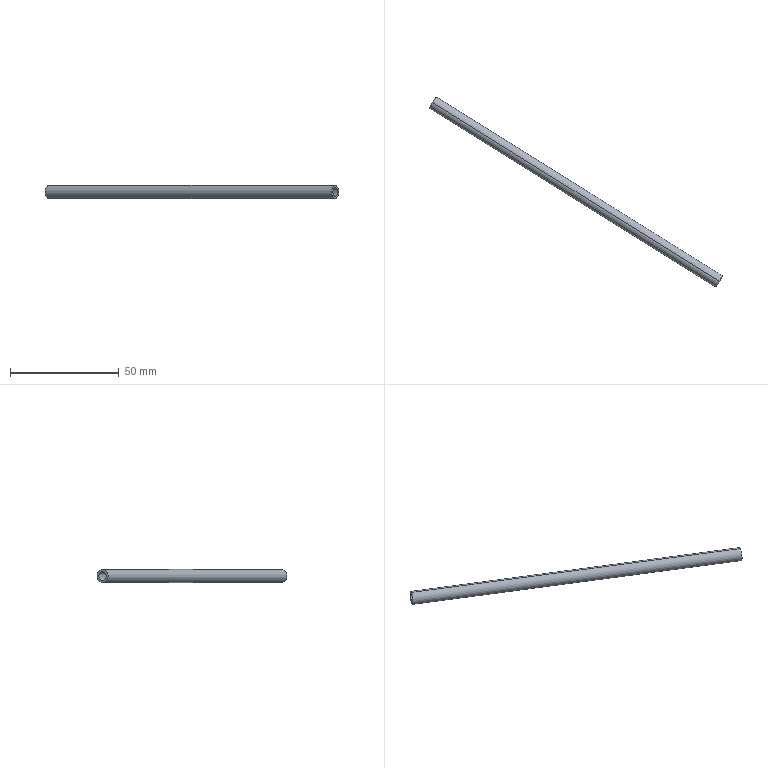Part | SolidWorks | features BaseBody 1 | 1 solid | 6 faces | box 134.627 x 87.226 x 6 mm | volume 2435 mm3 | cylinder 4 | plane 2 | commonest cylinder face diameters 4 x2 6 x2
STEP:
#1=CARTESIAN_POINT('',(-187.965,151.587,-231.5));
#2=VERTEX_POINT('',#1);
#3=CARTESIAN_POINT('',(-187.965,151.587,-235.5));
#4=VERTEX_POINT('',#3);
#5=CARTESIAN_POINT('',(-187.965,151.587,-233.5));
#6=DIRECTION('',(0.848,-0.5299,0.));
#7=DIRECTION('',(-0.5299,-0.848,0.));
#8=AXIS2_PLACEMENT_3D('',#5,#6,#7);
#9=CIRCLE('',#8,2.);
#10=EDGE_CURVE('',#2,#4,#9,.T.);
#11=ORIENTED_EDGE('',*,*,#10,.F.);
#12=CARTESIAN_POINT('',(-56.517,69.449,-231.5));
#13=VERTEX_POINT('',#12);
#14=CARTESIAN_POINT('',(-56.517,69.449,-231.5));
#15=DIRECTION('',(0.848,-0.5299,0.));
#16=VECTOR('',#15,1000.);
#17=LINE('',#14,#16);
#18=EDGE_CURVE('',#2,#13,#17,.T.);
#19=ORIENTED_EDGE('',*,*,#18,.T.);
#20=CARTESIAN_POINT('',(-56.517,69.449,-235.5));
#21=VERTEX_POINT('',#20);
#22=CARTESIAN_POINT('',(-56.517,69.449,-233.5));
#23=DIRECTION('',(0.848,-0.5299,0.));
#24=DIRECTION('',(0.,0.,-1.));
#25=AXIS2_PLACEMENT_3D('',#22,#23,#24);
#26=CIRCLE('',#25,2.);
#27=EDGE_CURVE('',#13,#21,#26,.T.);
#28=ORIENTED_EDGE('',*,*,#27,.T.);
#29=CARTESIAN_POINT('',(-56.517,69.449,-235.5));
#30=DIRECTION('',(0.848,-0.5299,0.));
#31=VECTOR('',#30,1000.);
#32=LINE('',#29,#31);
#33=EDGE_CURVE('',#4,#21,#32,.T.);
#34=ORIENTED_EDGE('',*,*,#33,.F.);
#35=EDGE_LOOP('',(#11,#19,#28,#34));
#36=FACE_OUTER_BOUND('',#35,.T.);
#37=CARTESIAN_POINT('',(-56.517,69.449,-233.5));
#38=DIRECTION('',(0.848,-0.5299,0.));
#39=DIRECTION('',(0.,0.,-1.));
#40=AXIS2_PLACEMENT_3D('',#37,#38,#39);
#41=CYLINDRICAL_SURFACE('',#40,2.);
#42=ADVANCED_FACE('',(#36),#41,.F.);
#43=CARTESIAN_POINT('',(-187.965,151.587,-236.5));
#44=VERTEX_POINT('',#43);
#45=CARTESIAN_POINT('',(-187.965,151.587,-230.5));
#46=VERTEX_POINT('',#45);
#47=CARTESIAN_POINT('',(-187.965,151.587,-233.5));
#48=DIRECTION('',(0.848,-0.5299,0.));
#49=DIRECTION('',(-0.5299,-0.848,0.));
#50=AXIS2_PLACEMENT_3D('',#47,#48,#49);
#51=CIRCLE('',#50,3.);
#52=EDGE_CURVE('',#44,#46,#51,.T.);
#53=ORIENTED_EDGE('',*,*,#52,.T.);
#54=CARTESIAN_POINT('',(-56.517,69.449,-230.5));
#55=VERTEX_POINT('',#54);
#56=CARTESIAN_POINT('',(-56.517,69.449,-230.5));
#57=DIRECTION('',(0.848,-0.5299,0.));
#58=VECTOR('',#57,1000.);
#59=LINE('',#56,#58);
#60=EDGE_CURVE('',#46,#55,#59,.T.);
#61=ORIENTED_EDGE('',*,*,#60,.T.);
#62=CARTESIAN_POINT('',(-56.517,69.449,-236.5));
#63=VERTEX_POINT('',#62);
#64=CARTESIAN_POINT('',(-56.517,69.449,-233.5));
#65=DIRECTION('',(0.848,-0.5299,0.));
#66=DIRECTION('',(0.,0.,-1.));
#67=AXIS2_PLACEMENT_3D('',#64,#65,#66);
#68=CIRCLE('',#67,3.);
#69=EDGE_CURVE('',#63,#55,#68,.T.);
#70=ORIENTED_EDGE('',*,*,#69,.F.);
#71=CARTESIAN_POINT('',(-56.517,69.449,-236.5));
#72=DIRECTION('',(0.848,-0.5299,0.));
#73=VECTOR('',#72,1000.);
#74=LINE('',#71,#73);
#75=EDGE_CURVE('',#44,#63,#74,.T.);
#76=ORIENTED_EDGE('',*,*,#75,.F.);
#77=EDGE_LOOP('',(#53,#61,#70,#76));
#78=FACE_OUTER_BOUND('',#77,.T.);
#79=CARTESIAN_POINT('',(-56.517,69.449,-233.5));
#80=DIRECTION('',(0.848,-0.5299,0.));
#81=DIRECTION('',(0.,0.,-1.));
#82=AXIS2_PLACEMENT_3D('',#79,#80,#81);
#83=CYLINDRICAL_SURFACE('',#82,3.);
#84=ADVANCED_FACE('',(#78),#83,.T.);
#85=ORIENTED_EDGE('',*,*,#60,.F.);
#86=CARTESIAN_POINT('',(-187.965,151.587,-233.5));
#87=DIRECTION('',(0.848,-0.5299,0.));
#88=DIRECTION('',(-0.5299,-0.848,0.));
#89=AXIS2_PLACEMENT_3D('',#86,#87,#88);
#90=CIRCLE('',#89,3.);
#91=EDGE_CURVE('',#46,#44,#90,.T.);
#92=ORIENTED_EDGE('',*,*,#91,.T.);
#93=ORIENTED_EDGE('',*,*,#75,.T.);
#94=CARTESIAN_POINT('',(-56.517,69.449,-233.5));
#95=DIRECTION('',(0.848,-0.5299,0.));
#96=DIRECTION('',(0.,0.,-1.));
#97=AXIS2_PLACEMENT_3D('',#94,#95,#96);
#98=CIRCLE('',#97,3.);
#99=EDGE_CURVE('',#55,#63,#98,.T.);
#100=ORIENTED_EDGE('',*,*,#99,.F.);
#101=EDGE_LOOP('',(#85,#92,#93,#100));
#102=FACE_OUTER_BOUND('',#101,.T.);
#103=CARTESIAN_POINT('',(-56.517,69.449,-233.5));
#104=DIRECTION('',(0.848,-0.5299,0.));
#105=DIRECTION('',(0.,0.,-1.));
#106=AXIS2_PLACEMENT_3D('',#103,#104,#105);
#107=CYLINDRICAL_SURFACE('',#106,3.);
#108=ADVANCED_FACE('',(#102),#107,.T.);
#109=CARTESIAN_POINT('',(-187.965,151.587,-233.5));
#110=DIRECTION('',(0.848,-0.5299,0.));
#111=DIRECTION('',(-0.5299,-0.848,0.));
#112=AXIS2_PLACEMENT_3D('',#109,#110,#111);
#113=CIRCLE('',#112,2.);
#114=EDGE_CURVE('',#4,#2,#113,.T.);
#115=ORIENTED_EDGE('',*,*,#114,.T.);
#116=ORIENTED_EDGE('',*,*,#10,.T.);
#117=EDGE_LOOP('',(#115,#116));
#118=FACE_BOUND('',#117,.T.);
#119=ORIENTED_EDGE('',*,*,#52,.F.);
#120=ORIENTED_EDGE('',*,*,#91,.F.);
#121=EDGE_LOOP('',(#119,#120));
#122=FACE_OUTER_BOUND('',#121,.T.);
#123=CARTESIAN_POINT('',(-186.375,154.131,-233.5));
#124=DIRECTION('',(-0.848,0.5299,0.));
#125=DIRECTION('',(0.,0.,1.));
#126=AXIS2_PLACEMENT_3D('',#123,#124,#125);
#127=PLANE('',#126);
#128=ADVANCED_FACE('',(#118,#122),#127,.T.);
#129=ORIENTED_EDGE('',*,*,#18,.F.);
#130=ORIENTED_EDGE('',*,*,#114,.F.);
#131=ORIENTED_EDGE('',*,*,#33,.T.);
#132=CARTESIAN_POINT('',(-56.517,69.449,-233.5));
#133=DIRECTION('',(0.848,-0.5299,0.));
#134=DIRECTION('',(0.,0.,-1.));
#135=AXIS2_PLACEMENT_3D('',#132,#133,#134);
#136=CIRCLE('',#135,2.);
#137=EDGE_CURVE('',#21,#13,#136,.T.);
#138=ORIENTED_EDGE('',*,*,#137,.T.);
#139=EDGE_LOOP('',(#129,#130,#131,#138));
#140=FACE_OUTER_BOUND('',#139,.T.);
#141=CARTESIAN_POINT('',(-56.517,69.449,-233.5));
#142=DIRECTION('',(0.848,-0.5299,0.));
#143=DIRECTION('',(0.,0.,-1.));
#144=AXIS2_PLACEMENT_3D('',#141,#142,#143);
#145=CYLINDRICAL_SURFACE('',#144,2.);
#146=ADVANCED_FACE('',(#140),#145,.F.);
#147=ORIENTED_EDGE('',*,*,#69,.T.);
#148=ORIENTED_EDGE('',*,*,#99,.T.);
#149=EDGE_LOOP('',(#147,#148));
#150=FACE_OUTER_BOUND('',#149,.T.);
#151=ORIENTED_EDGE('',*,*,#137,.F.);
#152=ORIENTED_EDGE('',*,*,#27,.F.);
#153=EDGE_LOOP('',(#151,#152));
#154=FACE_BOUND('',#153,.T.);
#155=CARTESIAN_POINT('',(-55.457,71.145,-233.5));
#156=DIRECTION('',(0.848,-0.5299,0.));
#157=DIRECTION('',(0.,0.,-1.));
#158=AXIS2_PLACEMENT_3D('',#155,#156,#157);
#159=PLANE('',#158);
#160=ADVANCED_FACE('',(#150,#154),#159,.T.);
#161=CLOSED_SHELL('',(#42,#84,#108,#128,#146,#160));
#162=MANIFOLD_SOLID_BREP('',#161);
#163=CARTESIAN_POINT('',(0.,0.,0.));
#164=DIRECTION('',(0.,0.,1.));
#165=DIRECTION('',(1.,0.,0.));
#166=AXIS2_PLACEMENT_3D('',#163,#164,#165);
#167=(LENGTH_UNIT()NAMED_UNIT(*)SI_UNIT(.MILLI.,.METRE.));
#168=UNCERTAINTY_MEASURE_WITH_UNIT(LENGTH_MEASURE(0.00001),#167,'','');
#169=(NAMED_UNIT(*)PLANE_ANGLE_UNIT()SI_UNIT($,.RADIAN.));
#170=(NAMED_UNIT(*)SI_UNIT($,.STERADIAN.)SOLID_ANGLE_UNIT());
#171=(GEOMETRIC_REPRESENTATION_CONTEXT(3)GLOBAL_UNCERTAINTY_ASSIGNED_CONTEXT((#168))GLOBAL_UNIT_ASSIGNED_CONTEXT((#167,#169,#170))REPRESENTATION_CONTEXT('',''));
#172=ADVANCED_BREP_SHAPE_REPRESENTATION('',(#162,#166),#171);